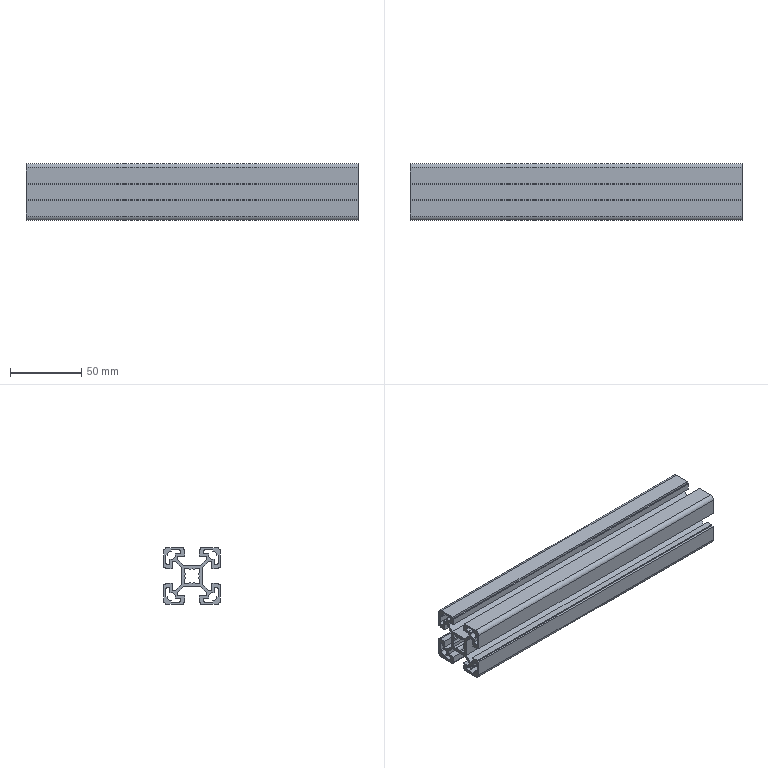Part | STEP file | AL PROFILE 4040 L 456 | 1 solid | 137 faces | box 233.35 x 40 x 40 mm | volume 129692 mm3 | plane 110 | cylinder 27 | commonest cylinder face diameters 3 x10 5.5 x8 10 x5 6 x4